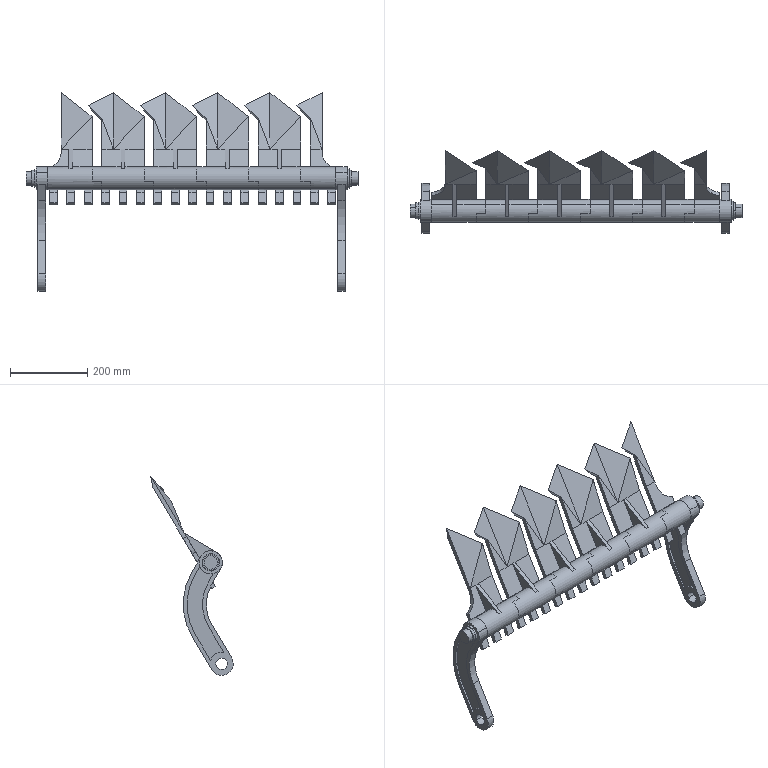Part | SolidWorks | features ReferencePattern 3, AEMSimFeature 1, LocalLPattern 1 | 12 solids | 456 faces | box 859 x 213.314 x 514.351 mm | volume 4241595 mm3 | plane 338 | cylinder 106 | torus 12 | commonest cylinder face diameters 60 x38 40 x18 12 x10 1.2 x8 35 x6 30 x4